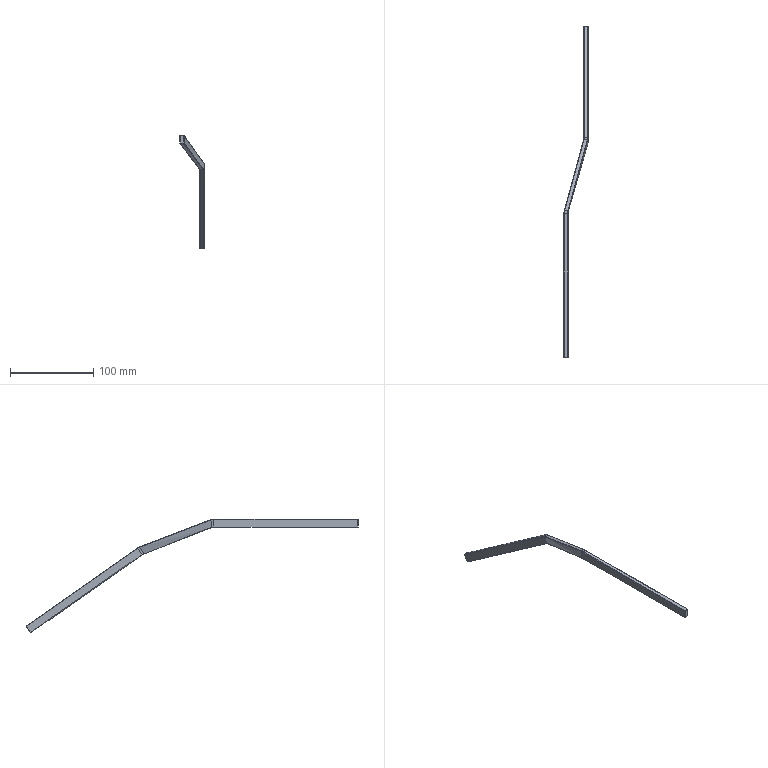Part | STEP file | ESG3 | 1 solid | 74 faces | box 29 x 398.586 x 136.529 mm | volume 21277 mm3 | spline 42 | cylinder 20 | plane 12 | commonest cylinder face diameters 1 x16 20 x4